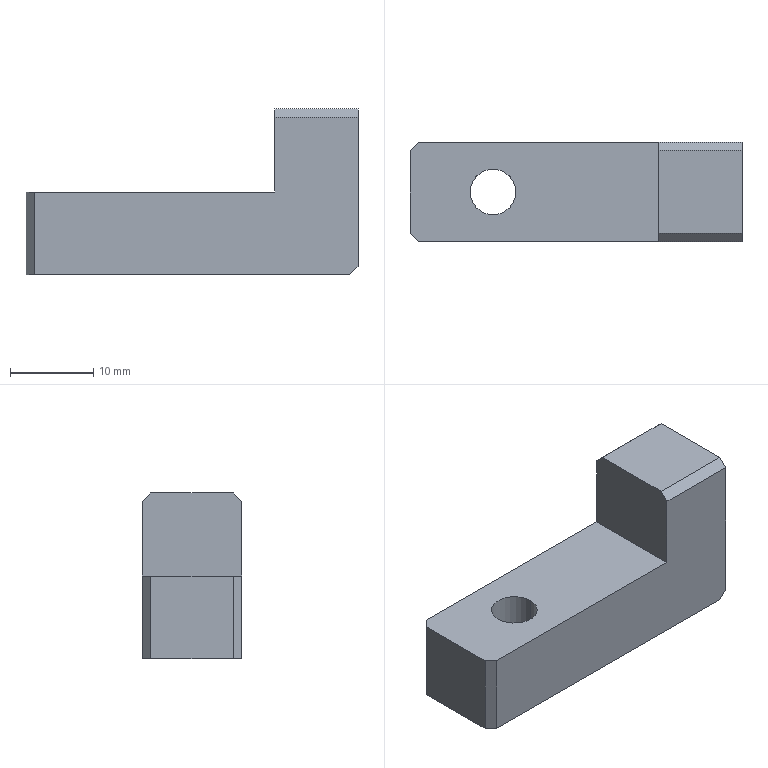Part | SolidWorks | features Chamfer 1, Extrusion 1, HoleWzd 1, ICE 1 | 1 solid | 18 faces | box 40 x 12 x 20 mm | volume 5424 mm3 | plane 14 | cylinder 4 | commonest cylinder face diameters 5.5 x2 10 x2
STEP:
#1=CARTESIAN_POINT('',(-5.,0.,-4.3));
#2=VERTEX_POINT('',#1);
#3=CARTESIAN_POINT('',(-15.,0.,-4.3));
#4=VERTEX_POINT('',#3);
#5=CARTESIAN_POINT('',(-10.,0.,-4.3));
#6=DIRECTION('',(0.,0.,-1.));
#7=DIRECTION('',(-1.,0.,0.));
#8=AXIS2_PLACEMENT_3D('',#5,#6,#7);
#9=CIRCLE('',#8,5.);
#10=EDGE_CURVE('',#2,#4,#9,.T.);
#11=ORIENTED_EDGE('',*,*,#10,.F.);
#12=CARTESIAN_POINT('',(-5.,0.,-10.));
#13=VERTEX_POINT('',#12);
#14=CARTESIAN_POINT('',(-5.,0.,-10.));
#15=DIRECTION('',(0.,0.,-1.));
#16=VECTOR('',#15,1000.);
#17=LINE('',#14,#16);
#18=EDGE_CURVE('',#2,#13,#17,.T.);
#19=ORIENTED_EDGE('',*,*,#18,.T.);
#20=CARTESIAN_POINT('',(-15.,0.,-10.));
#21=VERTEX_POINT('',#20);
#22=CARTESIAN_POINT('',(-10.,0.,-10.));
#23=DIRECTION('',(0.,0.,-1.));
#24=DIRECTION('',(-1.,0.,0.));
#25=AXIS2_PLACEMENT_3D('',#22,#23,#24);
#26=CIRCLE('',#25,5.);
#27=EDGE_CURVE('',#13,#21,#26,.T.);
#28=ORIENTED_EDGE('',*,*,#27,.T.);
#29=CARTESIAN_POINT('',(-15.,0.,-10.));
#30=DIRECTION('',(0.,0.,-1.));
#31=VECTOR('',#30,1000.);
#32=LINE('',#29,#31);
#33=EDGE_CURVE('',#4,#21,#32,.T.);
#34=ORIENTED_EDGE('',*,*,#33,.F.);
#35=EDGE_LOOP('',(#11,#19,#28,#34));
#36=FACE_OUTER_BOUND('',#35,.T.);
#37=CARTESIAN_POINT('',(-10.,0.,-10.));
#38=DIRECTION('',(0.,0.,-1.));
#39=DIRECTION('',(-1.,0.,0.));
#40=AXIS2_PLACEMENT_3D('',#37,#38,#39);
#41=CYLINDRICAL_SURFACE('',#40,5.);
#42=ADVANCED_FACE('',(#36),#41,.F.);
#43=CARTESIAN_POINT('',(-7.25,0.,0.));
#44=VERTEX_POINT('',#43);
#45=CARTESIAN_POINT('',(-12.75,0.,0.));
#46=VERTEX_POINT('',#45);
#47=CARTESIAN_POINT('',(-10.,0.,0.));
#48=DIRECTION('',(0.,0.,-1.));
#49=DIRECTION('',(-1.,0.,0.));
#50=AXIS2_PLACEMENT_3D('',#47,#48,#49);
#51=CIRCLE('',#50,2.75);
#52=EDGE_CURVE('',#44,#46,#51,.T.);
#53=ORIENTED_EDGE('',*,*,#52,.F.);
#54=CARTESIAN_POINT('',(-7.25,0.,-4.3));
#55=VERTEX_POINT('',#54);
#56=CARTESIAN_POINT('',(-7.25,0.,-10.));
#57=DIRECTION('',(0.,0.,-1.));
#58=VECTOR('',#57,1000.);
#59=LINE('',#56,#58);
#60=EDGE_CURVE('',#44,#55,#59,.T.);
#61=ORIENTED_EDGE('',*,*,#60,.T.);
#62=CARTESIAN_POINT('',(-12.75,0.,-4.3));
#63=VERTEX_POINT('',#62);
#64=CARTESIAN_POINT('',(-10.,0.,-4.3));
#65=DIRECTION('',(0.,0.,-1.));
#66=DIRECTION('',(-1.,0.,0.));
#67=AXIS2_PLACEMENT_3D('',#64,#65,#66);
#68=CIRCLE('',#67,2.75);
#69=EDGE_CURVE('',#55,#63,#68,.T.);
#70=ORIENTED_EDGE('',*,*,#69,.T.);
#71=CARTESIAN_POINT('',(-12.75,0.,-10.));
#72=DIRECTION('',(0.,0.,-1.));
#73=VECTOR('',#72,1000.);
#74=LINE('',#71,#73);
#75=EDGE_CURVE('',#46,#63,#74,.T.);
#76=ORIENTED_EDGE('',*,*,#75,.F.);
#77=EDGE_LOOP('',(#53,#61,#70,#76));
#78=FACE_OUTER_BOUND('',#77,.T.);
#79=CARTESIAN_POINT('',(-10.,0.,-10.));
#80=DIRECTION('',(0.,0.,-1.));
#81=DIRECTION('',(-1.,0.,0.));
#82=AXIS2_PLACEMENT_3D('',#79,#80,#81);
#83=CYLINDRICAL_SURFACE('',#82,2.75);
#84=ADVANCED_FACE('',(#78),#83,.F.);
#85=CARTESIAN_POINT('',(20.,6.,9.));
#86=VERTEX_POINT('',#85);
#87=CARTESIAN_POINT('',(20.,6.,-9.));
#88=VERTEX_POINT('',#87);
#89=CARTESIAN_POINT('',(20.,6.,10.));
#90=DIRECTION('',(0.,0.,-1.));
#91=VECTOR('',#90,1000.);
#92=LINE('',#89,#91);
#93=EDGE_CURVE('',#86,#88,#92,.T.);
#94=ORIENTED_EDGE('',*,*,#93,.F.);
#95=CARTESIAN_POINT('',(20.,5.,10.));
#96=VERTEX_POINT('',#95);
#97=CARTESIAN_POINT('',(20.,6.,9.));
#98=DIRECTION('',(0.,-0.7071,0.7071));
#99=VECTOR('',#98,1000.);
#100=LINE('',#97,#99);
#101=EDGE_CURVE('',#86,#96,#100,.T.);
#102=ORIENTED_EDGE('',*,*,#101,.T.);
#103=CARTESIAN_POINT('',(20.,-5.,10.));
#104=VERTEX_POINT('',#103);
#105=CARTESIAN_POINT('',(20.,6.,10.));
#106=DIRECTION('',(0.,-1.,0.));
#107=VECTOR('',#106,1000.);
#108=LINE('',#105,#107);
#109=EDGE_CURVE('',#96,#104,#108,.T.);
#110=ORIENTED_EDGE('',*,*,#109,.T.);
#111=CARTESIAN_POINT('',(20.,-6.,9.));
#112=VERTEX_POINT('',#111);
#113=CARTESIAN_POINT('',(20.,-5.,10.));
#114=DIRECTION('',(0.,-0.7071,-0.7071));
#115=VECTOR('',#114,1000.);
#116=LINE('',#113,#115);
#117=EDGE_CURVE('',#104,#112,#116,.T.);
#118=ORIENTED_EDGE('',*,*,#117,.T.);
#119=CARTESIAN_POINT('',(20.,-6.,-9.));
#120=VERTEX_POINT('',#119);
#121=CARTESIAN_POINT('',(20.,-6.,10.));
#122=DIRECTION('',(0.,0.,-1.));
#123=VECTOR('',#122,1000.);
#124=LINE('',#121,#123);
#125=EDGE_CURVE('',#112,#120,#124,.T.);
#126=ORIENTED_EDGE('',*,*,#125,.T.);
#127=CARTESIAN_POINT('',(20.,6.,-9.));
#128=DIRECTION('',(0.,1.,0.));
#129=VECTOR('',#128,1000.);
#130=LINE('',#127,#129);
#131=EDGE_CURVE('',#120,#88,#130,.T.);
#132=ORIENTED_EDGE('',*,*,#131,.T.);
#133=EDGE_LOOP('',(#94,#102,#110,#118,#126,#132));
#134=FACE_OUTER_BOUND('',#133,.T.);
#135=CARTESIAN_POINT('',(20.,6.,10.));
#136=DIRECTION('',(-1.,0.,0.));
#137=DIRECTION('',(0.,0.,1.));
#138=AXIS2_PLACEMENT_3D('',#135,#136,#137);
#139=PLANE('',#138);
#140=ADVANCED_FACE('',(#134),#139,.F.);
#141=CARTESIAN_POINT('',(-10.,0.,-10.));
#142=DIRECTION('',(0.,0.,-1.));
#143=DIRECTION('',(-1.,0.,0.));
#144=AXIS2_PLACEMENT_3D('',#141,#142,#143);
#145=CIRCLE('',#144,5.);
#146=EDGE_CURVE('',#21,#13,#145,.T.);
#147=ORIENTED_EDGE('',*,*,#146,.F.);
#148=ORIENTED_EDGE('',*,*,#27,.F.);
#149=EDGE_LOOP('',(#147,#148));
#150=FACE_BOUND('',#149,.T.);
#151=CARTESIAN_POINT('',(19.,6.,-10.));
#152=VERTEX_POINT('',#151);
#153=CARTESIAN_POINT('',(-19.,6.,-10.));
#154=VERTEX_POINT('',#153);
#155=CARTESIAN_POINT('',(-20.,6.,-10.));
#156=DIRECTION('',(-1.,0.,0.));
#157=VECTOR('',#156,1000.);
#158=LINE('',#155,#157);
#159=EDGE_CURVE('',#152,#154,#158,.T.);
#160=ORIENTED_EDGE('',*,*,#159,.F.);
#161=CARTESIAN_POINT('',(19.,-6.,-10.));
#162=VERTEX_POINT('',#161);
#163=CARTESIAN_POINT('',(19.,6.,-10.));
#164=DIRECTION('',(0.,-1.,0.));
#165=VECTOR('',#164,1000.);
#166=LINE('',#163,#165);
#167=EDGE_CURVE('',#152,#162,#166,.T.);
#168=ORIENTED_EDGE('',*,*,#167,.T.);
#169=CARTESIAN_POINT('',(-19.,-6.,-10.));
#170=VERTEX_POINT('',#169);
#171=CARTESIAN_POINT('',(-20.,-6.,-10.));
#172=DIRECTION('',(-1.,0.,0.));
#173=VECTOR('',#172,1000.);
#174=LINE('',#171,#173);
#175=EDGE_CURVE('',#162,#170,#174,.T.);
#176=ORIENTED_EDGE('',*,*,#175,.T.);
#177=CARTESIAN_POINT('',(-20.,-5.,-10.));
#178=VERTEX_POINT('',#177);
#179=CARTESIAN_POINT('',(-20.,-5.,-10.));
#180=DIRECTION('',(-0.7071,0.7071,0.));
#181=VECTOR('',#180,1000.);
#182=LINE('',#179,#181);
#183=EDGE_CURVE('',#170,#178,#182,.T.);
#184=ORIENTED_EDGE('',*,*,#183,.T.);
#185=CARTESIAN_POINT('',(-20.,5.,-10.));
#186=VERTEX_POINT('',#185);
#187=CARTESIAN_POINT('',(-20.,6.,-10.));
#188=DIRECTION('',(0.,-1.,0.));
#189=VECTOR('',#188,1000.);
#190=LINE('',#187,#189);
#191=EDGE_CURVE('',#186,#178,#190,.T.);
#192=ORIENTED_EDGE('',*,*,#191,.F.);
#193=CARTESIAN_POINT('',(-19.,6.,-10.));
#194=DIRECTION('',(0.7071,0.7071,0.));
#195=VECTOR('',#194,1000.);
#196=LINE('',#193,#195);
#197=EDGE_CURVE('',#186,#154,#196,.T.);
#198=ORIENTED_EDGE('',*,*,#197,.T.);
#199=EDGE_LOOP('',(#160,#168,#176,#184,#192,#198));
#200=FACE_OUTER_BOUND('',#199,.T.);
#201=CARTESIAN_POINT('',(-20.,6.,-10.));
#202=DIRECTION('',(0.,0.,1.));
#203=DIRECTION('',(1.,0.,0.));
#204=AXIS2_PLACEMENT_3D('',#201,#202,#203);
#205=PLANE('',#204);
#206=ADVANCED_FACE('',(#150,#200),#205,.F.);
#207=CARTESIAN_POINT('',(-20.,-5.,0.));
#208=VERTEX_POINT('',#207);
#209=CARTESIAN_POINT('',(-20.,5.,0.));
#210=VERTEX_POINT('',#209);
#211=CARTESIAN_POINT('',(-20.,-37.623,0.));
#212=DIRECTION('',(0.,1.,0.));
#213=VECTOR('',#212,1000.);
#214=LINE('',#211,#213);
#215=EDGE_CURVE('',#208,#210,#214,.T.);
#216=ORIENTED_EDGE('',*,*,#215,.T.);
#217=CARTESIAN_POINT('',(-20.,5.,10.));
#218=DIRECTION('',(0.,0.,-1.));
#219=VECTOR('',#218,1000.);
#220=LINE('',#217,#219);
#221=EDGE_CURVE('',#210,#186,#220,.T.);
#222=ORIENTED_EDGE('',*,*,#221,.T.);
#223=ORIENTED_EDGE('',*,*,#191,.T.);
#224=CARTESIAN_POINT('',(-20.,-5.,0.));
#225=DIRECTION('',(0.,0.,1.));
#226=VECTOR('',#225,1000.);
#227=LINE('',#224,#226);
#228=EDGE_CURVE('',#178,#208,#227,.T.);
#229=ORIENTED_EDGE('',*,*,#228,.T.);
#230=EDGE_LOOP('',(#216,#222,#223,#229));
#231=FACE_OUTER_BOUND('',#230,.T.);
#232=CARTESIAN_POINT('',(-20.,6.,10.));
#233=DIRECTION('',(1.,0.,0.));
#234=DIRECTION('',(0.,0.,-1.));
#235=AXIS2_PLACEMENT_3D('',#232,#233,#234);
#236=PLANE('',#235);
#237=ADVANCED_FACE('',(#231),#236,.F.);
#238=ORIENTED_EDGE('',*,*,#109,.F.);
#239=CARTESIAN_POINT('',(10.,5.,10.));
#240=VERTEX_POINT('',#239);
#241=CARTESIAN_POINT('',(-20.,5.,10.));
#242=DIRECTION('',(-1.,0.,0.));
#243=VECTOR('',#242,1000.);
#244=LINE('',#241,#243);
#245=EDGE_CURVE('',#96,#240,#244,.T.);
#246=ORIENTED_EDGE('',*,*,#245,.T.);
#247=CARTESIAN_POINT('',(10.,-5.,10.));
#248=VERTEX_POINT('',#247);
#249=CARTESIAN_POINT('',(10.,-37.623,10.));
#250=DIRECTION('',(0.,1.,0.));
#251=VECTOR('',#250,1000.);
#252=LINE('',#249,#251);
#253=EDGE_CURVE('',#248,#240,#252,.T.);
#254=ORIENTED_EDGE('',*,*,#253,.F.);
#255=CARTESIAN_POINT('',(20.,-5.,10.));
#256=DIRECTION('',(1.,0.,0.));
#257=VECTOR('',#256,1000.);
#258=LINE('',#255,#257);
#259=EDGE_CURVE('',#248,#104,#258,.T.);
#260=ORIENTED_EDGE('',*,*,#259,.T.);
#261=EDGE_LOOP('',(#238,#246,#254,#260));
#262=FACE_OUTER_BOUND('',#261,.T.);
#263=CARTESIAN_POINT('',(-20.,6.,10.));
#264=DIRECTION('',(0.,0.,-1.));
#265=DIRECTION('',(-1.,0.,0.));
#266=AXIS2_PLACEMENT_3D('',#263,#264,#265);
#267=PLANE('',#266);
#268=ADVANCED_FACE('',(#262),#267,.F.);
#269=CARTESIAN_POINT('',(10.,6.,9.));
#270=VERTEX_POINT('',#269);
#271=CARTESIAN_POINT('',(10.,6.,0.));
#272=VERTEX_POINT('',#271);
#273=CARTESIAN_POINT('',(10.,6.,10.));
#274=DIRECTION('',(0.,0.,-1.));
#275=VECTOR('',#274,1000.);
#276=LINE('',#273,#275);
#277=EDGE_CURVE('',#270,#272,#276,.T.);
#278=ORIENTED_EDGE('',*,*,#277,.F.);
#279=CARTESIAN_POINT('',(0.,6.,9.));
#280=DIRECTION('',(1.,0.,0.));
#281=VECTOR('',#280,1000.);
#282=LINE('',#279,#281);
#283=EDGE_CURVE('',#270,#86,#282,.T.);
#284=ORIENTED_EDGE('',*,*,#283,.T.);
#285=ORIENTED_EDGE('',*,*,#93,.T.);
#286=CARTESIAN_POINT('',(19.,6.,-10.));
#287=DIRECTION('',(-0.7071,0.,-0.7071));
#288=VECTOR('',#287,1000.);
#289=LINE('',#286,#288);
#290=EDGE_CURVE('',#88,#152,#289,.T.);
#291=ORIENTED_EDGE('',*,*,#290,.T.);
#292=ORIENTED_EDGE('',*,*,#159,.T.);
#293=CARTESIAN_POINT('',(-19.,6.,0.));
#294=VERTEX_POINT('',#293);
#295=CARTESIAN_POINT('',(-19.,6.,0.));
#296=DIRECTION('',(0.,0.,1.));
#297=VECTOR('',#296,1000.);
#298=LINE('',#295,#297);
#299=EDGE_CURVE('',#154,#294,#298,.T.);
#300=ORIENTED_EDGE('',*,*,#299,.T.);
#301=CARTESIAN_POINT('',(-20.,6.,0.));
#302=DIRECTION('',(-1.,0.,0.));
#303=VECTOR('',#302,1000.);
#304=LINE('',#301,#303);
#305=EDGE_CURVE('',#272,#294,#304,.T.);
#306=ORIENTED_EDGE('',*,*,#305,.F.);
#307=EDGE_LOOP('',(#278,#284,#285,#291,#292,#300,#306));
#308=FACE_OUTER_BOUND('',#307,.T.);
#309=CARTESIAN_POINT('',(0.,6.,0.));
#310=DIRECTION('',(0.,-1.,0.));
#311=DIRECTION('',(0.,0.,-1.));
#312=AXIS2_PLACEMENT_3D('',#309,#310,#311);
#313=PLANE('',#312);
#314=ADVANCED_FACE('',(#308),#313,.F.);
#315=ORIENTED_EDGE('',*,*,#125,.F.);
#316=CARTESIAN_POINT('',(10.,-6.,9.));
#317=VERTEX_POINT('',#316);
#318=CARTESIAN_POINT('',(10.,-6.,9.));
#319=DIRECTION('',(-1.,0.,0.));
#320=VECTOR('',#319,1000.);
#321=LINE('',#318,#320);
#322=EDGE_CURVE('',#112,#317,#321,.T.);
#323=ORIENTED_EDGE('',*,*,#322,.T.);
#324=CARTESIAN_POINT('',(10.,-6.,0.));
#325=VERTEX_POINT('',#324);
#326=CARTESIAN_POINT('',(10.,-6.,10.));
#327=DIRECTION('',(0.,0.,-1.));
#328=VECTOR('',#327,1000.);
#329=LINE('',#326,#328);
#330=EDGE_CURVE('',#317,#325,#329,.T.);
#331=ORIENTED_EDGE('',*,*,#330,.T.);
#332=CARTESIAN_POINT('',(-19.,-6.,0.));
#333=VERTEX_POINT('',#332);
#334=CARTESIAN_POINT('',(-20.,-6.,0.));
#335=DIRECTION('',(-1.,0.,0.));
#336=VECTOR('',#335,1000.);
#337=LINE('',#334,#336);
#338=EDGE_CURVE('',#325,#333,#337,.T.);
#339=ORIENTED_EDGE('',*,*,#338,.T.);
#340=CARTESIAN_POINT('',(-19.,-6.,-10.));
#341=DIRECTION('',(0.,0.,-1.));
#342=VECTOR('',#341,1000.);
#343=LINE('',#340,#342);
#344=EDGE_CURVE('',#333,#170,#343,.T.);
#345=ORIENTED_EDGE('',*,*,#344,.T.);
#346=ORIENTED_EDGE('',*,*,#175,.F.);
#347=CARTESIAN_POINT('',(14.5,-6.,-14.5));
#348=DIRECTION('',(0.7071,0.,0.7071));
#349=VECTOR('',#348,1000.);
#350=LINE('',#347,#349);
#351=EDGE_CURVE('',#162,#120,#350,.T.);
#352=ORIENTED_EDGE('',*,*,#351,.T.);
#353=EDGE_LOOP('',(#315,#323,#331,#339,#345,#346,#352));
#354=FACE_OUTER_BOUND('',#353,.T.);
#355=CARTESIAN_POINT('',(0.,-6.,0.));
#356=DIRECTION('',(0.,-1.,0.));
#357=DIRECTION('',(0.,0.,-1.));
#358=AXIS2_PLACEMENT_3D('',#355,#356,#357);
#359=PLANE('',#358);
#360=ADVANCED_FACE('',(#354),#359,.T.);
#361=ORIENTED_EDGE('',*,*,#253,.T.);
#362=CARTESIAN_POINT('',(10.,6.,9.));
#363=DIRECTION('',(0.,0.7071,-0.7071));
#364=VECTOR('',#363,1000.);
#365=LINE('',#362,#364);
#366=EDGE_CURVE('',#240,#270,#365,.T.);
#367=ORIENTED_EDGE('',*,*,#366,.T.);
#368=ORIENTED_EDGE('',*,*,#277,.T.);
#369=CARTESIAN_POINT('',(10.,-37.623,0.));
#370=DIRECTION('',(0.,1.,0.));
#371=VECTOR('',#370,1000.);
#372=LINE('',#369,#371);
#373=EDGE_CURVE('',#325,#272,#372,.T.);
#374=ORIENTED_EDGE('',*,*,#373,.F.);
#375=ORIENTED_EDGE('',*,*,#330,.F.);
#376=CARTESIAN_POINT('',(10.,-5.,10.));
#377=DIRECTION('',(0.,0.7071,0.7071));
#378=VECTOR('',#377,1000.);
#379=LINE('',#376,#378);
#380=EDGE_CURVE('',#317,#248,#379,.T.);
#381=ORIENTED_EDGE('',*,*,#380,.T.);
#382=EDGE_LOOP('',(#361,#367,#368,#374,#375,#381));
#383=FACE_OUTER_BOUND('',#382,.T.);
#384=CARTESIAN_POINT('',(10.,-37.623,10.));
#385=DIRECTION('',(1.,0.,0.));
#386=DIRECTION('',(0.,0.,-1.));
#387=AXIS2_PLACEMENT_3D('',#384,#385,#386);
#388=PLANE('',#387);
#389=ADVANCED_FACE('',(#383),#388,.F.);
#390=CARTESIAN_POINT('',(-10.,0.,0.));
#391=DIRECTION('',(0.,0.,-1.));
#392=DIRECTION('',(-1.,0.,0.));
#393=AXIS2_PLACEMENT_3D('',#390,#391,#392);
#394=CIRCLE('',#393,2.75);
#395=EDGE_CURVE('',#46,#44,#394,.T.);
#396=ORIENTED_EDGE('',*,*,#395,.T.);
#397=ORIENTED_EDGE('',*,*,#52,.T.);
#398=EDGE_LOOP('',(#396,#397));
#399=FACE_BOUND('',#398,.T.);
#400=ORIENTED_EDGE('',*,*,#305,.T.);
#401=CARTESIAN_POINT('',(-19.,6.,0.));
#402=DIRECTION('',(-0.7071,-0.7071,0.));
#403=VECTOR('',#402,1000.);
#404=LINE('',#401,#403);
#405=EDGE_CURVE('',#294,#210,#404,.T.);
#406=ORIENTED_EDGE('',*,*,#405,.T.);
#407=ORIENTED_EDGE('',*,*,#215,.F.);
#408=CARTESIAN_POINT('',(-20.,-5.,0.));
#409=DIRECTION('',(0.7071,-0.7071,0.));
#410=VECTOR('',#409,1000.);
#411=LINE('',#408,#410);
#412=EDGE_CURVE('',#208,#333,#411,.T.);
#413=ORIENTED_EDGE('',*,*,#412,.T.);
#414=ORIENTED_EDGE('',*,*,#338,.F.);
#415=ORIENTED_EDGE('',*,*,#373,.T.);
#416=EDGE_LOOP('',(#400,#406,#407,#413,#414,#415));
#417=FACE_OUTER_BOUND('',#416,.T.);
#418=CARTESIAN_POINT('',(-20.,-37.623,0.));
#419=DIRECTION('',(0.,0.,-1.));
#420=DIRECTION('',(-1.,0.,0.));
#421=AXIS2_PLACEMENT_3D('',#418,#419,#420);
#422=PLANE('',#421);
#423=ADVANCED_FACE('',(#399,#417),#422,.F.);
#424=ORIENTED_EDGE('',*,*,#60,.F.);
#425=ORIENTED_EDGE('',*,*,#395,.F.);
#426=ORIENTED_EDGE('',*,*,#75,.T.);
#427=CARTESIAN_POINT('',(-10.,0.,-4.3));
#428=DIRECTION('',(0.,0.,-1.));
#429=DIRECTION('',(-1.,0.,0.));
#430=AXIS2_PLACEMENT_3D('',#427,#428,#429);
#431=CIRCLE('',#430,2.75);
#432=EDGE_CURVE('',#63,#55,#431,.T.);
#433=ORIENTED_EDGE('',*,*,#432,.T.);
#434=EDGE_LOOP('',(#424,#425,#426,#433));
#435=FACE_OUTER_BOUND('',#434,.T.);
#436=CARTESIAN_POINT('',(-10.,0.,-10.));
#437=DIRECTION('',(0.,0.,-1.));
#438=DIRECTION('',(-1.,0.,0.));
#439=AXIS2_PLACEMENT_3D('',#436,#437,#438);
#440=CYLINDRICAL_SURFACE('',#439,2.75);
#441=ADVANCED_FACE('',(#435),#440,.F.);
#442=ORIENTED_EDGE('',*,*,#432,.F.);
#443=ORIENTED_EDGE('',*,*,#69,.F.);
#444=EDGE_LOOP('',(#442,#443));
#445=FACE_BOUND('',#444,.T.);
#446=CARTESIAN_POINT('',(-10.,0.,-4.3));
#447=DIRECTION('',(0.,0.,-1.));
#448=DIRECTION('',(-1.,0.,0.));
#449=AXIS2_PLACEMENT_3D('',#446,#447,#448);
#450=CIRCLE('',#449,5.);
#451=EDGE_CURVE('',#4,#2,#450,.T.);
#452=ORIENTED_EDGE('',*,*,#451,.T.);
#453=ORIENTED_EDGE('',*,*,#10,.T.);
#454=EDGE_LOOP('',(#452,#453));
#455=FACE_OUTER_BOUND('',#454,.T.);
#456=CARTESIAN_POINT('',(-7.25,0.,-4.3));
#457=DIRECTION('',(0.,0.,1.));
#458=DIRECTION('',(1.,0.,0.));
#459=AXIS2_PLACEMENT_3D('',#456,#457,#458);
#460=PLANE('',#459);
#461=ADVANCED_FACE('',(#445,#455),#460,.F.);
#462=ORIENTED_EDGE('',*,*,#18,.F.);
#463=ORIENTED_EDGE('',*,*,#451,.F.);
#464=ORIENTED_EDGE('',*,*,#33,.T.);
#465=ORIENTED_EDGE('',*,*,#146,.T.);
#466=EDGE_LOOP('',(#462,#463,#464,#465));
#467=FACE_OUTER_BOUND('',#466,.T.);
#468=CARTESIAN_POINT('',(-10.,0.,-10.));
#469=DIRECTION('',(0.,0.,-1.));
#470=DIRECTION('',(-1.,0.,0.));
#471=AXIS2_PLACEMENT_3D('',#468,#469,#470);
#472=CYLINDRICAL_SURFACE('',#471,5.);
#473=ADVANCED_FACE('',(#467),#472,.F.);
#474=ORIENTED_EDGE('',*,*,#366,.F.);
#475=ORIENTED_EDGE('',*,*,#245,.F.);
#476=ORIENTED_EDGE('',*,*,#101,.F.);
#477=ORIENTED_EDGE('',*,*,#283,.F.);
#478=EDGE_LOOP('',(#474,#475,#476,#477));
#479=FACE_OUTER_BOUND('',#478,.T.);
#480=CARTESIAN_POINT('',(0.,6.,9.));
#481=DIRECTION('',(0.,-0.7071,-0.7071));
#482=DIRECTION('',(1.,0.,0.));
#483=AXIS2_PLACEMENT_3D('',#480,#481,#482);
#484=PLANE('',#483);
#485=ADVANCED_FACE('',(#479),#484,.F.);
#486=ORIENTED_EDGE('',*,*,#380,.F.);
#487=ORIENTED_EDGE('',*,*,#322,.F.);
#488=ORIENTED_EDGE('',*,*,#117,.F.);
#489=ORIENTED_EDGE('',*,*,#259,.F.);
#490=EDGE_LOOP('',(#486,#487,#488,#489));
#491=FACE_OUTER_BOUND('',#490,.T.);
#492=CARTESIAN_POINT('',(-20.,-5.,10.));
#493=DIRECTION('',(0.,-0.7071,0.7071));
#494=DIRECTION('',(-1.,0.,0.));
#495=AXIS2_PLACEMENT_3D('',#492,#493,#494);
#496=PLANE('',#495);
#497=ADVANCED_FACE('',(#491),#496,.T.);
#498=ORIENTED_EDGE('',*,*,#290,.F.);
#499=ORIENTED_EDGE('',*,*,#131,.F.);
#500=ORIENTED_EDGE('',*,*,#351,.F.);
#501=ORIENTED_EDGE('',*,*,#167,.F.);
#502=EDGE_LOOP('',(#498,#499,#500,#501));
#503=FACE_OUTER_BOUND('',#502,.T.);
#504=CARTESIAN_POINT('',(19.,6.,-10.));
#505=DIRECTION('',(-0.7071,0.,0.7071));
#506=DIRECTION('',(0.,-1.,0.));
#507=AXIS2_PLACEMENT_3D('',#504,#505,#506);
#508=PLANE('',#507);
#509=ADVANCED_FACE('',(#503),#508,.F.);
#510=ORIENTED_EDGE('',*,*,#197,.F.);
#511=ORIENTED_EDGE('',*,*,#221,.F.);
#512=ORIENTED_EDGE('',*,*,#405,.F.);
#513=ORIENTED_EDGE('',*,*,#299,.F.);
#514=EDGE_LOOP('',(#510,#511,#512,#513));
#515=FACE_OUTER_BOUND('',#514,.T.);
#516=CARTESIAN_POINT('',(-19.,6.,0.));
#517=DIRECTION('',(0.7071,-0.7071,0.));
#518=DIRECTION('',(0.,0.,1.));
#519=AXIS2_PLACEMENT_3D('',#516,#517,#518);
#520=PLANE('',#519);
#521=ADVANCED_FACE('',(#515),#520,.F.);
#522=ORIENTED_EDGE('',*,*,#183,.F.);
#523=ORIENTED_EDGE('',*,*,#344,.F.);
#524=ORIENTED_EDGE('',*,*,#412,.F.);
#525=ORIENTED_EDGE('',*,*,#228,.F.);
#526=EDGE_LOOP('',(#522,#523,#524,#525));
#527=FACE_OUTER_BOUND('',#526,.T.);
#528=CARTESIAN_POINT('',(-20.,-5.,10.));
#529=DIRECTION('',(-0.7071,-0.7071,0.));
#530=DIRECTION('',(0.,0.,-1.));
#531=AXIS2_PLACEMENT_3D('',#528,#529,#530);
#532=PLANE('',#531);
#533=ADVANCED_FACE('',(#527),#532,.T.);
#534=CLOSED_SHELL('',(#42,#84,#140,#206,#237,#268,#314,#360,#389,#423,#441,#461,#473,#485,#497,#509,#521,#533));
#535=MANIFOLD_SOLID_BREP('',#534);
#536=CARTESIAN_POINT('',(0.,0.,0.));
#537=DIRECTION('',(0.,0.,1.));
#538=DIRECTION('',(1.,0.,0.));
#539=AXIS2_PLACEMENT_3D('',#536,#537,#538);
#540=(LENGTH_UNIT()NAMED_UNIT(*)SI_UNIT(.MILLI.,.METRE.));
#541=UNCERTAINTY_MEASURE_WITH_UNIT(LENGTH_MEASURE(0.00001),#540,'','');
#542=(NAMED_UNIT(*)PLANE_ANGLE_UNIT()SI_UNIT($,.RADIAN.));
#543=(NAMED_UNIT(*)SI_UNIT($,.STERADIAN.)SOLID_ANGLE_UNIT());
#544=(GEOMETRIC_REPRESENTATION_CONTEXT(3)GLOBAL_UNCERTAINTY_ASSIGNED_CONTEXT((#541))GLOBAL_UNIT_ASSIGNED_CONTEXT((#540,#542,#543))REPRESENTATION_CONTEXT('',''));
#545=ADVANCED_BREP_SHAPE_REPRESENTATION('',(#535,#539),#544);